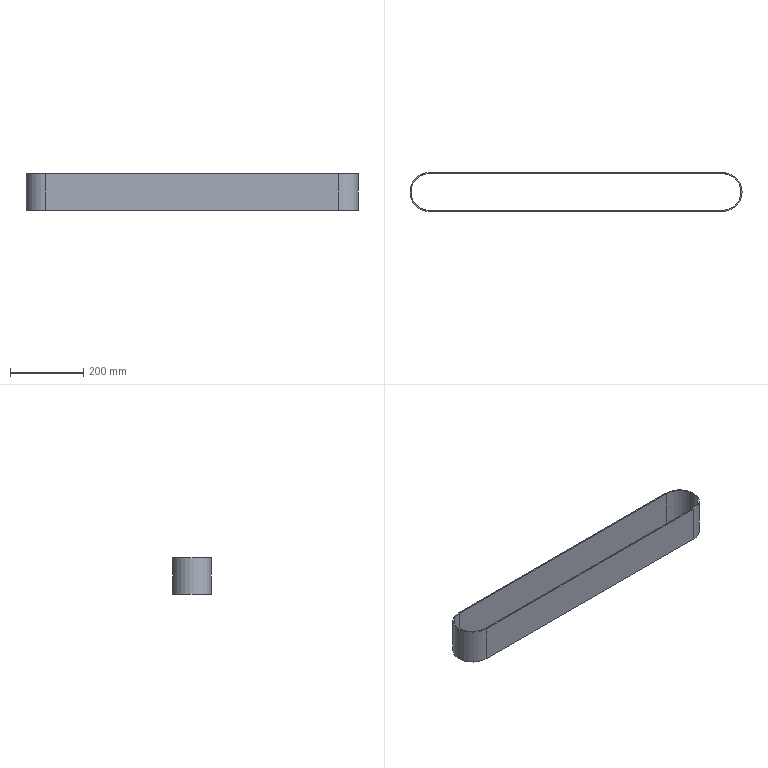Part | STEP file | 1 solid | 12 faces | box 906 x 106 x 100 mm | volume 577075 mm3 | cylinder 6 | plane 6 | commonest cylinder face diameters 100 x3 106 x3
STEP:
#1=CARTESIAN_POINT('',(0.,0.,0.));
#2=DIRECTION('',(0.,0.,1.));
#3=DIRECTION('',(1.,0.,0.));
#4=AXIS2_PLACEMENT_3D('',#1,#2,#3);
#5=CARTESIAN_POINT('',(640.53,56.408,0.));
#6=VERTEX_POINT('',#5);
#7=CARTESIAN_POINT('',(640.53,56.408,100.));
#8=VERTEX_POINT('',#7);
#9=CARTESIAN_POINT('',(640.53,56.408,0.));
#10=DIRECTION('',(0.,0.,1.));
#11=VECTOR('',#10,1.);
#12=LINE('',#9,#11);
#13=CARTESIAN_POINT('',(640.53,6.408,0.));
#14=DIRECTION('',(0.,0.,1.));
#15=DIRECTION('',(1.,0.,0.));
#16=AXIS2_PLACEMENT_3D('',#13,#14,#15);
#17=CYLINDRICAL_SURFACE('',#16,50.);
#18=CARTESIAN_POINT('',(1.571,0.));
#19=DIRECTION('',(0.,1.));
#20=VECTOR('',#19,1.);
#21=LINE('',#18,#20);
#22=(GEOMETRIC_REPRESENTATION_CONTEXT(2)PARAMETRIC_REPRESENTATION_CONTEXT()REPRESENTATION_CONTEXT('',''));
#23=DEFINITIONAL_REPRESENTATION('',(#21),#22);
#24=PCURVE('',#17,#23);
#25=CARTESIAN_POINT('',(640.53,56.408,0.));
#26=DIRECTION('',(0.,1.,0.));
#27=DIRECTION('',(0.,0.,1.));
#28=AXIS2_PLACEMENT_3D('',#25,#26,#27);
#29=PLANE('',#28);
#30=CARTESIAN_POINT('',(0.,0.));
#31=DIRECTION('',(1.,0.));
#32=VECTOR('',#31,1.);
#33=LINE('',#30,#32);
#34=(GEOMETRIC_REPRESENTATION_CONTEXT(2)PARAMETRIC_REPRESENTATION_CONTEXT()REPRESENTATION_CONTEXT('',''));
#35=DEFINITIONAL_REPRESENTATION('',(#33),#34);
#36=PCURVE('',#29,#35);
#37=SURFACE_CURVE('',#12,(#24,#36),.PCURVE_S1.);
#38=EDGE_CURVE('',#6,#8,#37,.T.);
#39=ORIENTED_EDGE('',*,*,#38,.T.);
#40=CARTESIAN_POINT('',(690.53,6.408,100.));
#41=VERTEX_POINT('',#40);
#42=CARTESIAN_POINT('',(640.53,6.408,100.));
#43=DIRECTION('',(0.,0.,-1.));
#44=DIRECTION('',(1.,0.,0.));
#45=AXIS2_PLACEMENT_3D('',#42,#43,#44);
#46=CIRCLE('',#45,50.);
#47=CARTESIAN_POINT('',(6.283,100.));
#48=DIRECTION('',(-1.,0.));
#49=VECTOR('',#48,1.);
#50=LINE('',#47,#49);
#51=(GEOMETRIC_REPRESENTATION_CONTEXT(2)PARAMETRIC_REPRESENTATION_CONTEXT()REPRESENTATION_CONTEXT('',''));
#52=DEFINITIONAL_REPRESENTATION('',(#50),#51);
#53=PCURVE('',#17,#52);
#54=CARTESIAN_POINT('',(240.531,6.408,100.));
#55=DIRECTION('',(0.,0.,1.));
#56=DIRECTION('',(1.,0.,0.));
#57=AXIS2_PLACEMENT_3D('',#54,#55,#56);
#58=PLANE('',#57);
#59=CARTESIAN_POINT('',(450.,0.));
#60=CARTESIAN_POINT('',(450.,-86.603));
#61=CARTESIAN_POINT('',(375.,-43.301));
#62=CARTESIAN_POINT('',(300.,0.));
#63=CARTESIAN_POINT('',(375.,43.301));
#64=CARTESIAN_POINT('',(450.,86.603));
#65=CARTESIAN_POINT('',(450.,0.));
#66=(BOUNDED_CURVE()B_SPLINE_CURVE(2,(#59,#60,#61,#62,#63,#64,#65),.UNSPECIFIED.,.T.,.F.)B_SPLINE_CURVE_WITH_KNOTS((1,2,2,2,2,1),(-2.094,0.,2.094,4.189,6.283,8.378),.UNSPECIFIED.)CURVE()GEOMETRIC_REPRESENTATION_ITEM()RATIONAL_B_SPLINE_CURVE((1.,0.5,1.,0.5,1.,0.5,1.))REPRESENTATION_ITEM(''));
#67=(GEOMETRIC_REPRESENTATION_CONTEXT(2)PARAMETRIC_REPRESENTATION_CONTEXT()REPRESENTATION_CONTEXT('',''));
#68=DEFINITIONAL_REPRESENTATION('',(#66),#67);
#69=PCURVE('',#58,#68);
#70=SURFACE_CURVE('',#46,(#53,#69),.PCURVE_S1.);
#71=EDGE_CURVE('',#8,#41,#70,.T.);
#72=ORIENTED_EDGE('',*,*,#71,.T.);
#73=CARTESIAN_POINT('',(690.53,6.408,0.));
#74=VERTEX_POINT('',#73);
#75=CARTESIAN_POINT('',(690.53,6.408,0.));
#76=DIRECTION('',(0.,0.,1.));
#77=VECTOR('',#76,1.);
#78=LINE('',#75,#77);
#79=CARTESIAN_POINT('',(0.,0.));
#80=DIRECTION('',(0.,1.));
#81=VECTOR('',#80,1.);
#82=LINE('',#79,#81);
#83=(GEOMETRIC_REPRESENTATION_CONTEXT(2)PARAMETRIC_REPRESENTATION_CONTEXT()REPRESENTATION_CONTEXT('',''));
#84=DEFINITIONAL_REPRESENTATION('',(#82),#83);
#85=PCURVE('',#17,#84);
#86=CARTESIAN_POINT('',(640.53,6.408,0.));
#87=DIRECTION('',(0.,0.,1.));
#88=DIRECTION('',(1.,0.,0.));
#89=AXIS2_PLACEMENT_3D('',#86,#87,#88);
#90=CYLINDRICAL_SURFACE('',#89,50.);
#91=CARTESIAN_POINT('',(6.283,0.));
#92=DIRECTION('',(0.,1.));
#93=VECTOR('',#92,1.);
#94=LINE('',#91,#93);
#95=(GEOMETRIC_REPRESENTATION_CONTEXT(2)PARAMETRIC_REPRESENTATION_CONTEXT()REPRESENTATION_CONTEXT('',''));
#96=DEFINITIONAL_REPRESENTATION('',(#94),#95);
#97=PCURVE('',#90,#96);
#98=SURFACE_CURVE('',#78,(#85,#97),.PCURVE_S1.);
#99=EDGE_CURVE('',#74,#41,#98,.T.);
#100=ORIENTED_EDGE('',*,*,#99,.F.);
#101=CARTESIAN_POINT('',(640.53,6.408,0.));
#102=DIRECTION('',(0.,0.,-1.));
#103=DIRECTION('',(1.,0.,0.));
#104=AXIS2_PLACEMENT_3D('',#101,#102,#103);
#105=CIRCLE('',#104,50.);
#106=CARTESIAN_POINT('',(6.283,0.));
#107=DIRECTION('',(-1.,0.));
#108=VECTOR('',#107,1.);
#109=LINE('',#106,#108);
#110=(GEOMETRIC_REPRESENTATION_CONTEXT(2)PARAMETRIC_REPRESENTATION_CONTEXT()REPRESENTATION_CONTEXT('',''));
#111=DEFINITIONAL_REPRESENTATION('',(#109),#110);
#112=PCURVE('',#17,#111);
#113=CARTESIAN_POINT('',(240.531,6.408,0.));
#114=DIRECTION('',(0.,0.,1.));
#115=DIRECTION('',(1.,0.,0.));
#116=AXIS2_PLACEMENT_3D('',#113,#114,#115);
#117=PLANE('',#116);
#118=CARTESIAN_POINT('',(450.,0.));
#119=CARTESIAN_POINT('',(450.,-86.603));
#120=CARTESIAN_POINT('',(375.,-43.301));
#121=CARTESIAN_POINT('',(300.,0.));
#122=CARTESIAN_POINT('',(375.,43.301));
#123=CARTESIAN_POINT('',(450.,86.603));
#124=CARTESIAN_POINT('',(450.,0.));
#125=(BOUNDED_CURVE()B_SPLINE_CURVE(2,(#118,#119,#120,#121,#122,#123,#124),.UNSPECIFIED.,.T.,.F.)B_SPLINE_CURVE_WITH_KNOTS((1,2,2,2,2,1),(-2.094,0.,2.094,4.189,6.283,8.378),.UNSPECIFIED.)CURVE()GEOMETRIC_REPRESENTATION_ITEM()RATIONAL_B_SPLINE_CURVE((1.,0.5,1.,0.5,1.,0.5,1.))REPRESENTATION_ITEM(''));
#126=(GEOMETRIC_REPRESENTATION_CONTEXT(2)PARAMETRIC_REPRESENTATION_CONTEXT()REPRESENTATION_CONTEXT('',''));
#127=DEFINITIONAL_REPRESENTATION('',(#125),#126);
#128=PCURVE('',#117,#127);
#129=SURFACE_CURVE('',#105,(#112,#128),.PCURVE_S1.);
#130=EDGE_CURVE('',#6,#74,#129,.T.);
#131=ORIENTED_EDGE('',*,*,#130,.F.);
#132=EDGE_LOOP('',(#39,#72,#100,#131));
#133=FACE_BOUND('',#132,.F.);
#134=ADVANCED_FACE('',(#133),#17,.F.);
#135=CARTESIAN_POINT('',(640.53,-46.592,0.));
#136=VERTEX_POINT('',#135);
#137=CARTESIAN_POINT('',(693.53,6.408,0.));
#138=VERTEX_POINT('',#137);
#139=CARTESIAN_POINT('',(640.53,6.408,0.));
#140=DIRECTION('',(0.,0.,1.));
#141=DIRECTION('',(1.,0.,0.));
#142=AXIS2_PLACEMENT_3D('',#139,#140,#141);
#143=CIRCLE('',#142,53.);
#144=CARTESIAN_POINT('',(640.53,6.408,0.));
#145=DIRECTION('',(0.,0.,1.));
#146=DIRECTION('',(1.,0.,0.));
#147=AXIS2_PLACEMENT_3D('',#144,#145,#146);
#148=CYLINDRICAL_SURFACE('',#147,53.);
#149=CARTESIAN_POINT('',(0.,0.));
#150=DIRECTION('',(1.,0.));
#151=VECTOR('',#150,1.);
#152=LINE('',#149,#151);
#153=(GEOMETRIC_REPRESENTATION_CONTEXT(2)PARAMETRIC_REPRESENTATION_CONTEXT()REPRESENTATION_CONTEXT('',''));
#154=DEFINITIONAL_REPRESENTATION('',(#152),#153);
#155=PCURVE('',#148,#154);
#156=CARTESIAN_POINT('',(400.,0.));
#157=DIRECTION('',(1.,0.));
#158=AXIS2_PLACEMENT_2D('',#156,#157);
#159=CIRCLE('',#158,53.);
#160=(GEOMETRIC_REPRESENTATION_CONTEXT(2)PARAMETRIC_REPRESENTATION_CONTEXT()REPRESENTATION_CONTEXT('',''));
#161=DEFINITIONAL_REPRESENTATION('',(#159),#160);
#162=PCURVE('',#117,#161);
#163=SURFACE_CURVE('',#143,(#155,#162),.PCURVE_S1.);
#164=EDGE_CURVE('',#136,#138,#163,.T.);
#165=ORIENTED_EDGE('',*,*,#164,.T.);
#166=CARTESIAN_POINT('',(693.53,6.408,100.));
#167=VERTEX_POINT('',#166);
#168=CARTESIAN_POINT('',(693.53,6.408,0.));
#169=DIRECTION('',(0.,0.,1.));
#170=VECTOR('',#169,1.);
#171=LINE('',#168,#170);
#172=CARTESIAN_POINT('',(6.283,0.));
#173=DIRECTION('',(0.,1.));
#174=VECTOR('',#173,1.);
#175=LINE('',#172,#174);
#176=(GEOMETRIC_REPRESENTATION_CONTEXT(2)PARAMETRIC_REPRESENTATION_CONTEXT()REPRESENTATION_CONTEXT('',''));
#177=DEFINITIONAL_REPRESENTATION('',(#175),#176);
#178=PCURVE('',#148,#177);
#179=CARTESIAN_POINT('',(640.53,6.408,0.));
#180=DIRECTION('',(0.,0.,1.));
#181=DIRECTION('',(1.,0.,0.));
#182=AXIS2_PLACEMENT_3D('',#179,#180,#181);
#183=CYLINDRICAL_SURFACE('',#182,53.);
#184=CARTESIAN_POINT('',(0.,0.));
#185=DIRECTION('',(0.,1.));
#186=VECTOR('',#185,1.);
#187=LINE('',#184,#186);
#188=(GEOMETRIC_REPRESENTATION_CONTEXT(2)PARAMETRIC_REPRESENTATION_CONTEXT()REPRESENTATION_CONTEXT('',''));
#189=DEFINITIONAL_REPRESENTATION('',(#187),#188);
#190=PCURVE('',#183,#189);
#191=SURFACE_CURVE('',#171,(#178,#190),.PCURVE_S1.);
#192=EDGE_CURVE('',#138,#167,#191,.T.);
#193=ORIENTED_EDGE('',*,*,#192,.T.);
#194=CARTESIAN_POINT('',(640.53,-46.592,100.));
#195=VERTEX_POINT('',#194);
#196=CARTESIAN_POINT('',(640.53,6.408,100.));
#197=DIRECTION('',(0.,0.,1.));
#198=DIRECTION('',(1.,0.,0.));
#199=AXIS2_PLACEMENT_3D('',#196,#197,#198);
#200=CIRCLE('',#199,53.);
#201=CARTESIAN_POINT('',(0.,100.));
#202=DIRECTION('',(1.,0.));
#203=VECTOR('',#202,1.);
#204=LINE('',#201,#203);
#205=(GEOMETRIC_REPRESENTATION_CONTEXT(2)PARAMETRIC_REPRESENTATION_CONTEXT()REPRESENTATION_CONTEXT('',''));
#206=DEFINITIONAL_REPRESENTATION('',(#204),#205);
#207=PCURVE('',#148,#206);
#208=CARTESIAN_POINT('',(400.,0.));
#209=DIRECTION('',(1.,0.));
#210=AXIS2_PLACEMENT_2D('',#208,#209);
#211=CIRCLE('',#210,53.);
#212=(GEOMETRIC_REPRESENTATION_CONTEXT(2)PARAMETRIC_REPRESENTATION_CONTEXT()REPRESENTATION_CONTEXT('',''));
#213=DEFINITIONAL_REPRESENTATION('',(#211),#212);
#214=PCURVE('',#58,#213);
#215=SURFACE_CURVE('',#200,(#207,#214),.PCURVE_S1.);
#216=EDGE_CURVE('',#195,#167,#215,.T.);
#217=ORIENTED_EDGE('',*,*,#216,.F.);
#218=CARTESIAN_POINT('',(640.53,-46.592,0.));
#219=DIRECTION('',(0.,0.,-1.));
#220=VECTOR('',#219,1.);
#221=LINE('',#218,#220);
#222=CARTESIAN_POINT('',(4.712,0.));
#223=DIRECTION('',(0.,-1.));
#224=VECTOR('',#223,1.);
#225=LINE('',#222,#224);
#226=(GEOMETRIC_REPRESENTATION_CONTEXT(2)PARAMETRIC_REPRESENTATION_CONTEXT()REPRESENTATION_CONTEXT('',''));
#227=DEFINITIONAL_REPRESENTATION('',(#225),#226);
#228=PCURVE('',#148,#227);
#229=CARTESIAN_POINT('',(-159.47,-46.592,0.));
#230=DIRECTION('',(0.,-1.,0.));
#231=DIRECTION('',(1.,0.,0.));
#232=AXIS2_PLACEMENT_3D('',#229,#230,#231);
#233=PLANE('',#232);
#234=CARTESIAN_POINT('',(800.,0.));
#235=DIRECTION('',(0.,-1.));
#236=VECTOR('',#235,1.);
#237=LINE('',#234,#236);
#238=(GEOMETRIC_REPRESENTATION_CONTEXT(2)PARAMETRIC_REPRESENTATION_CONTEXT()REPRESENTATION_CONTEXT('',''));
#239=DEFINITIONAL_REPRESENTATION('',(#237),#238);
#240=PCURVE('',#233,#239);
#241=SURFACE_CURVE('',#221,(#228,#240),.PCURVE_S1.);
#242=EDGE_CURVE('',#195,#136,#241,.T.);
#243=ORIENTED_EDGE('',*,*,#242,.T.);
#244=EDGE_LOOP('',(#165,#193,#217,#243));
#245=FACE_BOUND('',#244,.T.);
#246=ADVANCED_FACE('',(#245),#148,.T.);
#247=CARTESIAN_POINT('',(-159.47,-43.592,100.));
#248=VERTEX_POINT('',#247);
#249=CARTESIAN_POINT('',(-159.47,-43.592,0.));
#250=VERTEX_POINT('',#249);
#251=CARTESIAN_POINT('',(-159.47,-43.592,0.));
#252=DIRECTION('',(0.,0.,-1.));
#253=VECTOR('',#252,1.);
#254=LINE('',#251,#253);
#255=CARTESIAN_POINT('',(-159.47,-43.592,0.));
#256=DIRECTION('',(0.,-1.,0.));
#257=DIRECTION('',(1.,0.,0.));
#258=AXIS2_PLACEMENT_3D('',#255,#256,#257);
#259=PLANE('',#258);
#260=CARTESIAN_POINT('',(0.,0.));
#261=DIRECTION('',(0.,-1.));
#262=VECTOR('',#261,1.);
#263=LINE('',#260,#262);
#264=(GEOMETRIC_REPRESENTATION_CONTEXT(2)PARAMETRIC_REPRESENTATION_CONTEXT()REPRESENTATION_CONTEXT('',''));
#265=DEFINITIONAL_REPRESENTATION('',(#263),#264);
#266=PCURVE('',#259,#265);
#267=CARTESIAN_POINT('',(-159.47,6.408,0.));
#268=DIRECTION('',(0.,0.,1.));
#269=DIRECTION('',(1.,0.,0.));
#270=AXIS2_PLACEMENT_3D('',#267,#268,#269);
#271=CYLINDRICAL_SURFACE('',#270,50.);
#272=CARTESIAN_POINT('',(4.712,0.));
#273=DIRECTION('',(0.,-1.));
#274=VECTOR('',#273,1.);
#275=LINE('',#272,#274);
#276=(GEOMETRIC_REPRESENTATION_CONTEXT(2)PARAMETRIC_REPRESENTATION_CONTEXT()REPRESENTATION_CONTEXT('',''));
#277=DEFINITIONAL_REPRESENTATION('',(#275),#276);
#278=PCURVE('',#271,#277);
#279=SURFACE_CURVE('',#254,(#266,#278),.PCURVE_S1.);
#280=EDGE_CURVE('',#248,#250,#279,.T.);
#281=ORIENTED_EDGE('',*,*,#280,.F.);
#282=CARTESIAN_POINT('',(640.53,-43.592,100.));
#283=VERTEX_POINT('',#282);
#284=CARTESIAN_POINT('',(-159.47,-43.592,100.));
#285=DIRECTION('',(-1.,0.,0.));
#286=VECTOR('',#285,1.);
#287=LINE('',#284,#286);
#288=CARTESIAN_POINT('',(0.,100.));
#289=DIRECTION('',(-1.,0.));
#290=VECTOR('',#289,1.);
#291=LINE('',#288,#290);
#292=(GEOMETRIC_REPRESENTATION_CONTEXT(2)PARAMETRIC_REPRESENTATION_CONTEXT()REPRESENTATION_CONTEXT('',''));
#293=DEFINITIONAL_REPRESENTATION('',(#291),#292);
#294=PCURVE('',#259,#293);
#295=CARTESIAN_POINT('',(-400.,-50.));
#296=DIRECTION('',(-1.,0.));
#297=VECTOR('',#296,1.);
#298=LINE('',#295,#297);
#299=(GEOMETRIC_REPRESENTATION_CONTEXT(2)PARAMETRIC_REPRESENTATION_CONTEXT()REPRESENTATION_CONTEXT('',''));
#300=DEFINITIONAL_REPRESENTATION('',(#298),#299);
#301=PCURVE('',#58,#300);
#302=SURFACE_CURVE('',#287,(#294,#301),.PCURVE_S1.);
#303=EDGE_CURVE('',#283,#248,#302,.T.);
#304=ORIENTED_EDGE('',*,*,#303,.F.);
#305=CARTESIAN_POINT('',(640.53,-43.592,0.));
#306=VERTEX_POINT('',#305);
#307=CARTESIAN_POINT('',(640.53,-43.592,0.));
#308=DIRECTION('',(0.,0.,1.));
#309=VECTOR('',#308,1.);
#310=LINE('',#307,#309);
#311=CARTESIAN_POINT('',(800.,0.));
#312=DIRECTION('',(0.,1.));
#313=VECTOR('',#312,1.);
#314=LINE('',#311,#313);
#315=(GEOMETRIC_REPRESENTATION_CONTEXT(2)PARAMETRIC_REPRESENTATION_CONTEXT()REPRESENTATION_CONTEXT('',''));
#316=DEFINITIONAL_REPRESENTATION('',(#314),#315);
#317=PCURVE('',#259,#316);
#318=CARTESIAN_POINT('',(4.712,0.));
#319=DIRECTION('',(0.,1.));
#320=VECTOR('',#319,1.);
#321=LINE('',#318,#320);
#322=(GEOMETRIC_REPRESENTATION_CONTEXT(2)PARAMETRIC_REPRESENTATION_CONTEXT()REPRESENTATION_CONTEXT('',''));
#323=DEFINITIONAL_REPRESENTATION('',(#321),#322);
#324=PCURVE('',#90,#323);
#325=SURFACE_CURVE('',#310,(#317,#324),.PCURVE_S1.);
#326=EDGE_CURVE('',#306,#283,#325,.T.);
#327=ORIENTED_EDGE('',*,*,#326,.F.);
#328=CARTESIAN_POINT('',(-159.47,-43.592,0.));
#329=DIRECTION('',(1.,0.,0.));
#330=VECTOR('',#329,1.);
#331=LINE('',#328,#330);
#332=CARTESIAN_POINT('',(0.,0.));
#333=DIRECTION('',(1.,0.));
#334=VECTOR('',#333,1.);
#335=LINE('',#332,#334);
#336=(GEOMETRIC_REPRESENTATION_CONTEXT(2)PARAMETRIC_REPRESENTATION_CONTEXT()REPRESENTATION_CONTEXT('',''));
#337=DEFINITIONAL_REPRESENTATION('',(#335),#336);
#338=PCURVE('',#259,#337);
#339=CARTESIAN_POINT('',(-400.,-50.));
#340=DIRECTION('',(1.,0.));
#341=VECTOR('',#340,1.);
#342=LINE('',#339,#341);
#343=(GEOMETRIC_REPRESENTATION_CONTEXT(2)PARAMETRIC_REPRESENTATION_CONTEXT()REPRESENTATION_CONTEXT('',''));
#344=DEFINITIONAL_REPRESENTATION('',(#342),#343);
#345=PCURVE('',#117,#344);
#346=SURFACE_CURVE('',#331,(#338,#345),.PCURVE_S1.);
#347=EDGE_CURVE('',#250,#306,#346,.T.);
#348=ORIENTED_EDGE('',*,*,#347,.F.);
#349=EDGE_LOOP('',(#281,#304,#327,#348));
#350=FACE_BOUND('',#349,.T.);
#351=ADVANCED_FACE('',(#350),#259,.F.);
#352=ORIENTED_EDGE('',*,*,#164,.F.);
#353=CARTESIAN_POINT('',(-159.47,-46.592,0.));
#354=VERTEX_POINT('',#353);
#355=CARTESIAN_POINT('',(240.531,-46.592,0.));
#356=DIRECTION('',(1.,0.,0.));
#357=VECTOR('',#356,1.);
#358=LINE('',#355,#357);
#359=CARTESIAN_POINT('',(0.,-53.));
#360=DIRECTION('',(1.,0.));
#361=VECTOR('',#360,1.);
#362=LINE('',#359,#361);
#363=(GEOMETRIC_REPRESENTATION_CONTEXT(2)PARAMETRIC_REPRESENTATION_CONTEXT()REPRESENTATION_CONTEXT('',''));
#364=DEFINITIONAL_REPRESENTATION('',(#362),#363);
#365=PCURVE('',#117,#364);
#366=CARTESIAN_POINT('',(400.,0.));
#367=DIRECTION('',(1.,0.));
#368=VECTOR('',#367,1.);
#369=LINE('',#366,#368);
#370=(GEOMETRIC_REPRESENTATION_CONTEXT(2)PARAMETRIC_REPRESENTATION_CONTEXT()REPRESENTATION_CONTEXT('',''));
#371=DEFINITIONAL_REPRESENTATION('',(#369),#370);
#372=PCURVE('',#233,#371);
#373=SURFACE_CURVE('',#358,(#365,#372),.PCURVE_S1.);
#374=EDGE_CURVE('',#354,#136,#373,.T.);
#375=ORIENTED_EDGE('',*,*,#374,.F.);
#376=CARTESIAN_POINT('',(-159.47,59.408,0.));
#377=VERTEX_POINT('',#376);
#378=CARTESIAN_POINT('',(-159.47,6.408,0.));
#379=DIRECTION('',(0.,0.,1.));
#380=DIRECTION('',(1.,0.,0.));
#381=AXIS2_PLACEMENT_3D('',#378,#379,#380);
#382=CIRCLE('',#381,53.);
#383=CARTESIAN_POINT('',(-400.,0.));
#384=DIRECTION('',(1.,0.));
#385=AXIS2_PLACEMENT_2D('',#383,#384);
#386=CIRCLE('',#385,53.);
#387=(GEOMETRIC_REPRESENTATION_CONTEXT(2)PARAMETRIC_REPRESENTATION_CONTEXT()REPRESENTATION_CONTEXT('',''));
#388=DEFINITIONAL_REPRESENTATION('',(#386),#387);
#389=PCURVE('',#117,#388);
#390=CARTESIAN_POINT('',(-159.47,6.408,0.));
#391=DIRECTION('',(0.,0.,1.));
#392=DIRECTION('',(1.,0.,0.));
#393=AXIS2_PLACEMENT_3D('',#390,#391,#392);
#394=CYLINDRICAL_SURFACE('',#393,53.);
#395=CARTESIAN_POINT('',(0.,0.));
#396=DIRECTION('',(1.,0.));
#397=VECTOR('',#396,1.);
#398=LINE('',#395,#397);
#399=(GEOMETRIC_REPRESENTATION_CONTEXT(2)PARAMETRIC_REPRESENTATION_CONTEXT()REPRESENTATION_CONTEXT('',''));
#400=DEFINITIONAL_REPRESENTATION('',(#398),#399);
#401=PCURVE('',#394,#400);
#402=SURFACE_CURVE('',#382,(#389,#401),.PCURVE_S1.);
#403=EDGE_CURVE('',#377,#354,#402,.T.);
#404=ORIENTED_EDGE('',*,*,#403,.F.);
#405=CARTESIAN_POINT('',(640.53,59.408,0.));
#406=VERTEX_POINT('',#405);
#407=CARTESIAN_POINT('',(240.531,59.408,0.));
#408=DIRECTION('',(-1.,0.,0.));
#409=VECTOR('',#408,1.);
#410=LINE('',#407,#409);
#411=CARTESIAN_POINT('',(0.,53.));
#412=DIRECTION('',(-1.,0.));
#413=VECTOR('',#412,1.);
#414=LINE('',#411,#413);
#415=(GEOMETRIC_REPRESENTATION_CONTEXT(2)PARAMETRIC_REPRESENTATION_CONTEXT()REPRESENTATION_CONTEXT('',''));
#416=DEFINITIONAL_REPRESENTATION('',(#414),#415);
#417=PCURVE('',#117,#416);
#418=CARTESIAN_POINT('',(640.53,59.408,0.));
#419=DIRECTION('',(0.,1.,0.));
#420=DIRECTION('',(-1.,0.,0.));
#421=AXIS2_PLACEMENT_3D('',#418,#419,#420);
#422=PLANE('',#421);
#423=CARTESIAN_POINT('',(400.,0.));
#424=DIRECTION('',(1.,0.));
#425=VECTOR('',#424,1.);
#426=LINE('',#423,#425);
#427=(GEOMETRIC_REPRESENTATION_CONTEXT(2)PARAMETRIC_REPRESENTATION_CONTEXT()REPRESENTATION_CONTEXT('',''));
#428=DEFINITIONAL_REPRESENTATION('',(#426),#427);
#429=PCURVE('',#422,#428);
#430=SURFACE_CURVE('',#410,(#417,#429),.PCURVE_S1.);
#431=EDGE_CURVE('',#406,#377,#430,.T.);
#432=ORIENTED_EDGE('',*,*,#431,.F.);
#433=CARTESIAN_POINT('',(640.53,6.408,0.));
#434=DIRECTION('',(0.,0.,1.));
#435=DIRECTION('',(1.,0.,0.));
#436=AXIS2_PLACEMENT_3D('',#433,#434,#435);
#437=CIRCLE('',#436,53.);
#438=CARTESIAN_POINT('',(400.,0.));
#439=DIRECTION('',(1.,0.));
#440=AXIS2_PLACEMENT_2D('',#438,#439);
#441=CIRCLE('',#440,53.);
#442=(GEOMETRIC_REPRESENTATION_CONTEXT(2)PARAMETRIC_REPRESENTATION_CONTEXT()REPRESENTATION_CONTEXT('',''));
#443=DEFINITIONAL_REPRESENTATION('',(#441),#442);
#444=PCURVE('',#117,#443);
#445=CARTESIAN_POINT('',(0.,0.));
#446=DIRECTION('',(1.,0.));
#447=VECTOR('',#446,1.);
#448=LINE('',#445,#447);
#449=(GEOMETRIC_REPRESENTATION_CONTEXT(2)PARAMETRIC_REPRESENTATION_CONTEXT()REPRESENTATION_CONTEXT('',''));
#450=DEFINITIONAL_REPRESENTATION('',(#448),#449);
#451=PCURVE('',#183,#450);
#452=SURFACE_CURVE('',#437,(#444,#451),.PCURVE_S1.);
#453=EDGE_CURVE('',#138,#406,#452,.T.);
#454=ORIENTED_EDGE('',*,*,#453,.F.);
#455=EDGE_LOOP('',(#352,#375,#404,#432,#454));
#456=FACE_BOUND('',#455,.T.);
#457=CARTESIAN_POINT('',(-159.47,56.408,0.));
#458=VERTEX_POINT('',#457);
#459=CARTESIAN_POINT('',(240.531,56.408,0.));
#460=DIRECTION('',(1.,0.,0.));
#461=VECTOR('',#460,1.);
#462=LINE('',#459,#461);
#463=CARTESIAN_POINT('',(0.,50.));
#464=DIRECTION('',(1.,0.));
#465=VECTOR('',#464,1.);
#466=LINE('',#463,#465);
#467=(GEOMETRIC_REPRESENTATION_CONTEXT(2)PARAMETRIC_REPRESENTATION_CONTEXT()REPRESENTATION_CONTEXT('',''));
#468=DEFINITIONAL_REPRESENTATION('',(#466),#467);
#469=PCURVE('',#117,#468);
#470=CARTESIAN_POINT('',(0.,-400.));
#471=DIRECTION('',(0.,1.));
#472=VECTOR('',#471,1.);
#473=LINE('',#470,#472);
#474=(GEOMETRIC_REPRESENTATION_CONTEXT(2)PARAMETRIC_REPRESENTATION_CONTEXT()REPRESENTATION_CONTEXT('',''));
#475=DEFINITIONAL_REPRESENTATION('',(#473),#474);
#476=PCURVE('',#29,#475);
#477=SURFACE_CURVE('',#462,(#469,#476),.PCURVE_S1.);
#478=EDGE_CURVE('',#458,#6,#477,.T.);
#479=ORIENTED_EDGE('',*,*,#478,.F.);
#480=CARTESIAN_POINT('',(-159.47,6.408,0.));
#481=DIRECTION('',(0.,0.,-1.));
#482=DIRECTION('',(1.,0.,0.));
#483=AXIS2_PLACEMENT_3D('',#480,#481,#482);
#484=CIRCLE('',#483,50.);
#485=CARTESIAN_POINT('',(-350.,0.));
#486=CARTESIAN_POINT('',(-350.,-86.603));
#487=CARTESIAN_POINT('',(-425.,-43.301));
#488=CARTESIAN_POINT('',(-500.,0.));
#489=CARTESIAN_POINT('',(-425.,43.301));
#490=CARTESIAN_POINT('',(-350.,86.603));
#491=CARTESIAN_POINT('',(-350.,0.));
#492=(BOUNDED_CURVE()B_SPLINE_CURVE(2,(#485,#486,#487,#488,#489,#490,#491),.UNSPECIFIED.,.T.,.F.)B_SPLINE_CURVE_WITH_KNOTS((1,2,2,2,2,1),(-2.094,0.,2.094,4.189,6.283,8.378),.UNSPECIFIED.)CURVE()GEOMETRIC_REPRESENTATION_ITEM()RATIONAL_B_SPLINE_CURVE((1.,0.5,1.,0.5,1.,0.5,1.))REPRESENTATION_ITEM(''));
#493=(GEOMETRIC_REPRESENTATION_CONTEXT(2)PARAMETRIC_REPRESENTATION_CONTEXT()REPRESENTATION_CONTEXT('',''));
#494=DEFINITIONAL_REPRESENTATION('',(#492),#493);
#495=PCURVE('',#117,#494);
#496=CARTESIAN_POINT('',(6.283,0.));
#497=DIRECTION('',(-1.,0.));
#498=VECTOR('',#497,1.);
#499=LINE('',#496,#498);
#500=(GEOMETRIC_REPRESENTATION_CONTEXT(2)PARAMETRIC_REPRESENTATION_CONTEXT()REPRESENTATION_CONTEXT('',''));
#501=DEFINITIONAL_REPRESENTATION('',(#499),#500);
#502=PCURVE('',#271,#501);
#503=SURFACE_CURVE('',#484,(#495,#502),.PCURVE_S1.);
#504=EDGE_CURVE('',#250,#458,#503,.T.);
#505=ORIENTED_EDGE('',*,*,#504,.F.);
#506=ORIENTED_EDGE('',*,*,#347,.T.);
#507=CARTESIAN_POINT('',(640.53,6.408,0.));
#508=DIRECTION('',(0.,0.,-1.));
#509=DIRECTION('',(1.,0.,0.));
#510=AXIS2_PLACEMENT_3D('',#507,#508,#509);
#511=CIRCLE('',#510,50.);
#512=CARTESIAN_POINT('',(450.,0.));
#513=CARTESIAN_POINT('',(450.,-86.603));
#514=CARTESIAN_POINT('',(375.,-43.301));
#515=CARTESIAN_POINT('',(300.,0.));
#516=CARTESIAN_POINT('',(375.,43.301));
#517=CARTESIAN_POINT('',(450.,86.603));
#518=CARTESIAN_POINT('',(450.,0.));
#519=(BOUNDED_CURVE()B_SPLINE_CURVE(2,(#512,#513,#514,#515,#516,#517,#518),.UNSPECIFIED.,.T.,.F.)B_SPLINE_CURVE_WITH_KNOTS((1,2,2,2,2,1),(-2.094,0.,2.094,4.189,6.283,8.378),.UNSPECIFIED.)CURVE()GEOMETRIC_REPRESENTATION_ITEM()RATIONAL_B_SPLINE_CURVE((1.,0.5,1.,0.5,1.,0.5,1.))REPRESENTATION_ITEM(''));
#520=(GEOMETRIC_REPRESENTATION_CONTEXT(2)PARAMETRIC_REPRESENTATION_CONTEXT()REPRESENTATION_CONTEXT('',''));
#521=DEFINITIONAL_REPRESENTATION('',(#519),#520);
#522=PCURVE('',#117,#521);
#523=CARTESIAN_POINT('',(6.283,0.));
#524=DIRECTION('',(-1.,0.));
#525=VECTOR('',#524,1.);
#526=LINE('',#523,#525);
#527=(GEOMETRIC_REPRESENTATION_CONTEXT(2)PARAMETRIC_REPRESENTATION_CONTEXT()REPRESENTATION_CONTEXT('',''));
#528=DEFINITIONAL_REPRESENTATION('',(#526),#527);
#529=PCURVE('',#90,#528);
#530=SURFACE_CURVE('',#511,(#522,#529),.PCURVE_S1.);
#531=EDGE_CURVE('',#74,#306,#530,.T.);
#532=ORIENTED_EDGE('',*,*,#531,.F.);
#533=ORIENTED_EDGE('',*,*,#130,.F.);
#534=EDGE_LOOP('',(#479,#505,#506,#532,#533));
#535=FACE_BOUND('',#534,.T.);
#536=ADVANCED_FACE('',(#456,#535),#117,.F.);
#537=ORIENTED_EDGE('',*,*,#504,.F.);
#538=ORIENTED_EDGE('',*,*,#280,.F.);
#539=CARTESIAN_POINT('',(-159.47,56.408,100.));
#540=VERTEX_POINT('',#539);
#541=CARTESIAN_POINT('',(-159.47,6.408,100.));
#542=DIRECTION('',(0.,0.,-1.));
#543=DIRECTION('',(1.,0.,0.));
#544=AXIS2_PLACEMENT_3D('',#541,#542,#543);
#545=CIRCLE('',#544,50.);
#546=CARTESIAN_POINT('',(6.283,100.));
#547=DIRECTION('',(-1.,0.));
#548=VECTOR('',#547,1.);
#549=LINE('',#546,#548);
#550=(GEOMETRIC_REPRESENTATION_CONTEXT(2)PARAMETRIC_REPRESENTATION_CONTEXT()REPRESENTATION_CONTEXT('',''));
#551=DEFINITIONAL_REPRESENTATION('',(#549),#550);
#552=PCURVE('',#271,#551);
#553=CARTESIAN_POINT('',(-350.,0.));
#554=CARTESIAN_POINT('',(-350.,-86.603));
#555=CARTESIAN_POINT('',(-425.,-43.301));
#556=CARTESIAN_POINT('',(-500.,0.));
#557=CARTESIAN_POINT('',(-425.,43.301));
#558=CARTESIAN_POINT('',(-350.,86.603));
#559=CARTESIAN_POINT('',(-350.,0.));
#560=(BOUNDED_CURVE()B_SPLINE_CURVE(2,(#553,#554,#555,#556,#557,#558,#559),.UNSPECIFIED.,.T.,.F.)B_SPLINE_CURVE_WITH_KNOTS((1,2,2,2,2,1),(-2.094,0.,2.094,4.189,6.283,8.378),.UNSPECIFIED.)CURVE()GEOMETRIC_REPRESENTATION_ITEM()RATIONAL_B_SPLINE_CURVE((1.,0.5,1.,0.5,1.,0.5,1.))REPRESENTATION_ITEM(''));
#561=(GEOMETRIC_REPRESENTATION_CONTEXT(2)PARAMETRIC_REPRESENTATION_CONTEXT()REPRESENTATION_CONTEXT('',''));
#562=DEFINITIONAL_REPRESENTATION('',(#560),#561);
#563=PCURVE('',#58,#562);
#564=SURFACE_CURVE('',#545,(#552,#563),.PCURVE_S1.);
#565=EDGE_CURVE('',#248,#540,#564,.T.);
#566=ORIENTED_EDGE('',*,*,#565,.T.);
#567=CARTESIAN_POINT('',(-159.47,56.408,0.));
#568=DIRECTION('',(0.,0.,-1.));
#569=VECTOR('',#568,1.);
#570=LINE('',#567,#569);
#571=CARTESIAN_POINT('',(1.571,0.));
#572=DIRECTION('',(0.,-1.));
#573=VECTOR('',#572,1.);
#574=LINE('',#571,#573);
#575=(GEOMETRIC_REPRESENTATION_CONTEXT(2)PARAMETRIC_REPRESENTATION_CONTEXT()REPRESENTATION_CONTEXT('',''));
#576=DEFINITIONAL_REPRESENTATION('',(#574),#575);
#577=PCURVE('',#271,#576);
#578=CARTESIAN_POINT('',(0.,-800.));
#579=DIRECTION('',(-1.,0.));
#580=VECTOR('',#579,1.);
#581=LINE('',#578,#580);
#582=(GEOMETRIC_REPRESENTATION_CONTEXT(2)PARAMETRIC_REPRESENTATION_CONTEXT()REPRESENTATION_CONTEXT('',''));
#583=DEFINITIONAL_REPRESENTATION('',(#581),#582);
#584=PCURVE('',#29,#583);
#585=SURFACE_CURVE('',#570,(#577,#584),.PCURVE_S1.);
#586=EDGE_CURVE('',#540,#458,#585,.T.);
#587=ORIENTED_EDGE('',*,*,#586,.T.);
#588=EDGE_LOOP('',(#537,#538,#566,#587));
#589=FACE_BOUND('',#588,.F.);
#590=ADVANCED_FACE('',(#589),#271,.F.);
#591=CARTESIAN_POINT('',(-159.47,-46.592,100.));
#592=VERTEX_POINT('',#591);
#593=CARTESIAN_POINT('',(240.531,-46.592,100.));
#594=DIRECTION('',(1.,0.,0.));
#595=VECTOR('',#594,1.);
#596=LINE('',#593,#595);
#597=CARTESIAN_POINT('',(0.,-53.));
#598=DIRECTION('',(1.,0.));
#599=VECTOR('',#598,1.);
#600=LINE('',#597,#599);
#601=(GEOMETRIC_REPRESENTATION_CONTEXT(2)PARAMETRIC_REPRESENTATION_CONTEXT()REPRESENTATION_CONTEXT('',''));
#602=DEFINITIONAL_REPRESENTATION('',(#600),#601);
#603=PCURVE('',#58,#602);
#604=CARTESIAN_POINT('',(400.,100.));
#605=DIRECTION('',(1.,0.));
#606=VECTOR('',#605,1.);
#607=LINE('',#604,#606);
#608=(GEOMETRIC_REPRESENTATION_CONTEXT(2)PARAMETRIC_REPRESENTATION_CONTEXT()REPRESENTATION_CONTEXT('',''));
#609=DEFINITIONAL_REPRESENTATION('',(#607),#608);
#610=PCURVE('',#233,#609);
#611=SURFACE_CURVE('',#596,(#603,#610),.PCURVE_S1.);
#612=EDGE_CURVE('',#592,#195,#611,.T.);
#613=ORIENTED_EDGE('',*,*,#612,.T.);
#614=ORIENTED_EDGE('',*,*,#216,.T.);
#615=CARTESIAN_POINT('',(640.53,59.408,100.));
#616=VERTEX_POINT('',#615);
#617=CARTESIAN_POINT('',(640.53,6.408,100.));
#618=DIRECTION('',(0.,0.,1.));
#619=DIRECTION('',(1.,0.,0.));
#620=AXIS2_PLACEMENT_3D('',#617,#618,#619);
#621=CIRCLE('',#620,53.);
#622=CARTESIAN_POINT('',(400.,0.));
#623=DIRECTION('',(1.,0.));
#624=AXIS2_PLACEMENT_2D('',#622,#623);
#625=CIRCLE('',#624,53.);
#626=(GEOMETRIC_REPRESENTATION_CONTEXT(2)PARAMETRIC_REPRESENTATION_CONTEXT()REPRESENTATION_CONTEXT('',''));
#627=DEFINITIONAL_REPRESENTATION('',(#625),#626);
#628=PCURVE('',#58,#627);
#629=CARTESIAN_POINT('',(0.,100.));
#630=DIRECTION('',(1.,0.));
#631=VECTOR('',#630,1.);
#632=LINE('',#629,#631);
#633=(GEOMETRIC_REPRESENTATION_CONTEXT(2)PARAMETRIC_REPRESENTATION_CONTEXT()REPRESENTATION_CONTEXT('',''));
#634=DEFINITIONAL_REPRESENTATION('',(#632),#633);
#635=PCURVE('',#183,#634);
#636=SURFACE_CURVE('',#621,(#628,#635),.PCURVE_S1.);
#637=EDGE_CURVE('',#167,#616,#636,.T.);
#638=ORIENTED_EDGE('',*,*,#637,.T.);
#639=CARTESIAN_POINT('',(-159.47,59.408,100.));
#640=VERTEX_POINT('',#639);
#641=CARTESIAN_POINT('',(240.531,59.408,100.));
#642=DIRECTION('',(-1.,0.,0.));
#643=VECTOR('',#642,1.);
#644=LINE('',#641,#643);
#645=CARTESIAN_POINT('',(0.,53.));
#646=DIRECTION('',(-1.,0.));
#647=VECTOR('',#646,1.);
#648=LINE('',#645,#647);
#649=(GEOMETRIC_REPRESENTATION_CONTEXT(2)PARAMETRIC_REPRESENTATION_CONTEXT()REPRESENTATION_CONTEXT('',''));
#650=DEFINITIONAL_REPRESENTATION('',(#648),#649);
#651=PCURVE('',#58,#650);
#652=CARTESIAN_POINT('',(400.,100.));
#653=DIRECTION('',(1.,0.));
#654=VECTOR('',#653,1.);
#655=LINE('',#652,#654);
#656=(GEOMETRIC_REPRESENTATION_CONTEXT(2)PARAMETRIC_REPRESENTATION_CONTEXT()REPRESENTATION_CONTEXT('',''));
#657=DEFINITIONAL_REPRESENTATION('',(#655),#656);
#658=PCURVE('',#422,#657);
#659=SURFACE_CURVE('',#644,(#651,#658),.PCURVE_S1.);
#660=EDGE_CURVE('',#616,#640,#659,.T.);
#661=ORIENTED_EDGE('',*,*,#660,.T.);
#662=CARTESIAN_POINT('',(-159.47,6.408,100.));
#663=DIRECTION('',(0.,0.,1.));
#664=DIRECTION('',(1.,0.,0.));
#665=AXIS2_PLACEMENT_3D('',#662,#663,#664);
#666=CIRCLE('',#665,53.);
#667=CARTESIAN_POINT('',(-400.,0.));
#668=DIRECTION('',(1.,0.));
#669=AXIS2_PLACEMENT_2D('',#667,#668);
#670=CIRCLE('',#669,53.);
#671=(GEOMETRIC_REPRESENTATION_CONTEXT(2)PARAMETRIC_REPRESENTATION_CONTEXT()REPRESENTATION_CONTEXT('',''));
#672=DEFINITIONAL_REPRESENTATION('',(#670),#671);
#673=PCURVE('',#58,#672);
#674=CARTESIAN_POINT('',(0.,100.));
#675=DIRECTION('',(1.,0.));
#676=VECTOR('',#675,1.);
#677=LINE('',#674,#676);
#678=(GEOMETRIC_REPRESENTATION_CONTEXT(2)PARAMETRIC_REPRESENTATION_CONTEXT()REPRESENTATION_CONTEXT('',''));
#679=DEFINITIONAL_REPRESENTATION('',(#677),#678);
#680=PCURVE('',#394,#679);
#681=SURFACE_CURVE('',#666,(#673,#680),.PCURVE_S1.);
#682=EDGE_CURVE('',#640,#592,#681,.T.);
#683=ORIENTED_EDGE('',*,*,#682,.T.);
#684=EDGE_LOOP('',(#613,#614,#638,#661,#683));
#685=FACE_BOUND('',#684,.T.);
#686=ORIENTED_EDGE('',*,*,#565,.T.);
#687=CARTESIAN_POINT('',(240.531,56.408,100.));
#688=DIRECTION('',(1.,0.,0.));
#689=VECTOR('',#688,1.);
#690=LINE('',#687,#689);
#691=CARTESIAN_POINT('',(0.,50.));
#692=DIRECTION('',(1.,0.));
#693=VECTOR('',#692,1.);
#694=LINE('',#691,#693);
#695=(GEOMETRIC_REPRESENTATION_CONTEXT(2)PARAMETRIC_REPRESENTATION_CONTEXT()REPRESENTATION_CONTEXT('',''));
#696=DEFINITIONAL_REPRESENTATION('',(#694),#695);
#697=PCURVE('',#58,#696);
#698=CARTESIAN_POINT('',(100.,-400.));
#699=DIRECTION('',(0.,1.));
#700=VECTOR('',#699,1.);
#701=LINE('',#698,#700);
#702=(GEOMETRIC_REPRESENTATION_CONTEXT(2)PARAMETRIC_REPRESENTATION_CONTEXT()REPRESENTATION_CONTEXT('',''));
#703=DEFINITIONAL_REPRESENTATION('',(#701),#702);
#704=PCURVE('',#29,#703);
#705=SURFACE_CURVE('',#690,(#697,#704),.PCURVE_S1.);
#706=EDGE_CURVE('',#540,#8,#705,.T.);
#707=ORIENTED_EDGE('',*,*,#706,.T.);
#708=ORIENTED_EDGE('',*,*,#71,.T.);
#709=CARTESIAN_POINT('',(640.53,6.408,100.));
#710=DIRECTION('',(0.,0.,-1.));
#711=DIRECTION('',(1.,0.,0.));
#712=AXIS2_PLACEMENT_3D('',#709,#710,#711);
#713=CIRCLE('',#712,50.);
#714=CARTESIAN_POINT('',(450.,0.));
#715=CARTESIAN_POINT('',(450.,-86.603));
#716=CARTESIAN_POINT('',(375.,-43.301));
#717=CARTESIAN_POINT('',(300.,0.));
#718=CARTESIAN_POINT('',(375.,43.301));
#719=CARTESIAN_POINT('',(450.,86.603));
#720=CARTESIAN_POINT('',(450.,0.));
#721=(BOUNDED_CURVE()B_SPLINE_CURVE(2,(#714,#715,#716,#717,#718,#719,#720),.UNSPECIFIED.,.T.,.F.)B_SPLINE_CURVE_WITH_KNOTS((1,2,2,2,2,1),(-2.094,0.,2.094,4.189,6.283,8.378),.UNSPECIFIED.)CURVE()GEOMETRIC_REPRESENTATION_ITEM()RATIONAL_B_SPLINE_CURVE((1.,0.5,1.,0.5,1.,0.5,1.))REPRESENTATION_ITEM(''));
#722=(GEOMETRIC_REPRESENTATION_CONTEXT(2)PARAMETRIC_REPRESENTATION_CONTEXT()REPRESENTATION_CONTEXT('',''));
#723=DEFINITIONAL_REPRESENTATION('',(#721),#722);
#724=PCURVE('',#58,#723);
#725=CARTESIAN_POINT('',(6.283,100.));
#726=DIRECTION('',(-1.,0.));
#727=VECTOR('',#726,1.);
#728=LINE('',#725,#727);
#729=(GEOMETRIC_REPRESENTATION_CONTEXT(2)PARAMETRIC_REPRESENTATION_CONTEXT()REPRESENTATION_CONTEXT('',''));
#730=DEFINITIONAL_REPRESENTATION('',(#728),#729);
#731=PCURVE('',#90,#730);
#732=SURFACE_CURVE('',#713,(#724,#731),.PCURVE_S1.);
#733=EDGE_CURVE('',#41,#283,#732,.T.);
#734=ORIENTED_EDGE('',*,*,#733,.T.);
#735=ORIENTED_EDGE('',*,*,#303,.T.);
#736=EDGE_LOOP('',(#686,#707,#708,#734,#735));
#737=FACE_BOUND('',#736,.T.);
#738=ADVANCED_FACE('',(#685,#737),#58,.T.);
#739=ORIENTED_EDGE('',*,*,#733,.T.);
#740=ORIENTED_EDGE('',*,*,#326,.F.);
#741=ORIENTED_EDGE('',*,*,#531,.F.);
#742=ORIENTED_EDGE('',*,*,#99,.T.);
#743=EDGE_LOOP('',(#739,#740,#741,#742));
#744=FACE_BOUND('',#743,.F.);
#745=ADVANCED_FACE('',(#744),#90,.F.);
#746=ORIENTED_EDGE('',*,*,#660,.F.);
#747=CARTESIAN_POINT('',(640.53,59.408,0.));
#748=DIRECTION('',(0.,0.,-1.));
#749=VECTOR('',#748,1.);
#750=LINE('',#747,#749);
#751=CARTESIAN_POINT('',(0.,0.));
#752=DIRECTION('',(0.,-1.));
#753=VECTOR('',#752,1.);
#754=LINE('',#751,#753);
#755=(GEOMETRIC_REPRESENTATION_CONTEXT(2)PARAMETRIC_REPRESENTATION_CONTEXT()REPRESENTATION_CONTEXT('',''));
#756=DEFINITIONAL_REPRESENTATION('',(#754),#755);
#757=PCURVE('',#422,#756);
#758=CARTESIAN_POINT('',(1.571,0.));
#759=DIRECTION('',(0.,-1.));
#760=VECTOR('',#759,1.);
#761=LINE('',#758,#760);
#762=(GEOMETRIC_REPRESENTATION_CONTEXT(2)PARAMETRIC_REPRESENTATION_CONTEXT()REPRESENTATION_CONTEXT('',''));
#763=DEFINITIONAL_REPRESENTATION('',(#761),#762);
#764=PCURVE('',#183,#763);
#765=SURFACE_CURVE('',#750,(#757,#764),.PCURVE_S1.);
#766=EDGE_CURVE('',#616,#406,#765,.T.);
#767=ORIENTED_EDGE('',*,*,#766,.T.);
#768=ORIENTED_EDGE('',*,*,#431,.T.);
#769=CARTESIAN_POINT('',(-159.47,59.408,0.));
#770=DIRECTION('',(0.,0.,1.));
#771=VECTOR('',#770,1.);
#772=LINE('',#769,#771);
#773=CARTESIAN_POINT('',(800.,0.));
#774=DIRECTION('',(0.,1.));
#775=VECTOR('',#774,1.);
#776=LINE('',#773,#775);
#777=(GEOMETRIC_REPRESENTATION_CONTEXT(2)PARAMETRIC_REPRESENTATION_CONTEXT()REPRESENTATION_CONTEXT('',''));
#778=DEFINITIONAL_REPRESENTATION('',(#776),#777);
#779=PCURVE('',#422,#778);
#780=CARTESIAN_POINT('',(1.571,0.));
#781=DIRECTION('',(0.,1.));
#782=VECTOR('',#781,1.);
#783=LINE('',#780,#782);
#784=(GEOMETRIC_REPRESENTATION_CONTEXT(2)PARAMETRIC_REPRESENTATION_CONTEXT()REPRESENTATION_CONTEXT('',''));
#785=DEFINITIONAL_REPRESENTATION('',(#783),#784);
#786=PCURVE('',#394,#785);
#787=SURFACE_CURVE('',#772,(#779,#786),.PCURVE_S1.);
#788=EDGE_CURVE('',#377,#640,#787,.T.);
#789=ORIENTED_EDGE('',*,*,#788,.T.);
#790=EDGE_LOOP('',(#746,#767,#768,#789));
#791=FACE_BOUND('',#790,.T.);
#792=ADVANCED_FACE('',(#791),#422,.T.);
#793=ORIENTED_EDGE('',*,*,#192,.F.);
#794=ORIENTED_EDGE('',*,*,#453,.T.);
#795=ORIENTED_EDGE('',*,*,#766,.F.);
#796=ORIENTED_EDGE('',*,*,#637,.F.);
#797=EDGE_LOOP('',(#793,#794,#795,#796));
#798=FACE_BOUND('',#797,.T.);
#799=ADVANCED_FACE('',(#798),#183,.T.);
#800=ORIENTED_EDGE('',*,*,#612,.F.);
#801=CARTESIAN_POINT('',(-159.47,-46.592,0.));
#802=DIRECTION('',(0.,0.,-1.));
#803=VECTOR('',#802,1.);
#804=LINE('',#801,#803);
#805=CARTESIAN_POINT('',(0.,0.));
#806=DIRECTION('',(0.,-1.));
#807=VECTOR('',#806,1.);
#808=LINE('',#805,#807);
#809=(GEOMETRIC_REPRESENTATION_CONTEXT(2)PARAMETRIC_REPRESENTATION_CONTEXT()REPRESENTATION_CONTEXT('',''));
#810=DEFINITIONAL_REPRESENTATION('',(#808),#809);
#811=PCURVE('',#233,#810);
#812=CARTESIAN_POINT('',(4.712,0.));
#813=DIRECTION('',(0.,-1.));
#814=VECTOR('',#813,1.);
#815=LINE('',#812,#814);
#816=(GEOMETRIC_REPRESENTATION_CONTEXT(2)PARAMETRIC_REPRESENTATION_CONTEXT()REPRESENTATION_CONTEXT('',''));
#817=DEFINITIONAL_REPRESENTATION('',(#815),#816);
#818=PCURVE('',#394,#817);
#819=SURFACE_CURVE('',#804,(#811,#818),.PCURVE_S1.);
#820=EDGE_CURVE('',#592,#354,#819,.T.);
#821=ORIENTED_EDGE('',*,*,#820,.T.);
#822=ORIENTED_EDGE('',*,*,#374,.T.);
#823=ORIENTED_EDGE('',*,*,#242,.F.);
#824=EDGE_LOOP('',(#800,#821,#822,#823));
#825=FACE_BOUND('',#824,.T.);
#826=ADVANCED_FACE('',(#825),#233,.T.);
#827=ORIENTED_EDGE('',*,*,#682,.F.);
#828=ORIENTED_EDGE('',*,*,#788,.F.);
#829=ORIENTED_EDGE('',*,*,#403,.T.);
#830=ORIENTED_EDGE('',*,*,#820,.F.);
#831=EDGE_LOOP('',(#827,#828,#829,#830));
#832=FACE_BOUND('',#831,.T.);
#833=ADVANCED_FACE('',(#832),#394,.T.);
#834=ORIENTED_EDGE('',*,*,#38,.T.);
#835=ORIENTED_EDGE('',*,*,#706,.F.);
#836=ORIENTED_EDGE('',*,*,#586,.T.);
#837=ORIENTED_EDGE('',*,*,#478,.T.);
#838=EDGE_LOOP('',(#834,#835,#836,#837));
#839=FACE_BOUND('',#838,.T.);
#840=ADVANCED_FACE('',(#839),#29,.F.);
#841=CLOSED_SHELL('',(#134,#246,#351,#536,#590,#738,#745,#792,#799,#826,#833,#840));
#842=MANIFOLD_SOLID_BREP('',#841);
#843=(LENGTH_UNIT()NAMED_UNIT(*)SI_UNIT(.MILLI.,.METRE.));
#844=UNCERTAINTY_MEASURE_WITH_UNIT(LENGTH_MEASURE(0.0000001),#843,'','');
#845=(NAMED_UNIT(*)PLANE_ANGLE_UNIT()SI_UNIT($,.RADIAN.));
#846=(NAMED_UNIT(*)SI_UNIT($,.STERADIAN.)SOLID_ANGLE_UNIT());
#847=(GEOMETRIC_REPRESENTATION_CONTEXT(3)GLOBAL_UNCERTAINTY_ASSIGNED_CONTEXT((#844))GLOBAL_UNIT_ASSIGNED_CONTEXT((#843,#845,#846))REPRESENTATION_CONTEXT('',''));
#848=ADVANCED_BREP_SHAPE_REPRESENTATION('',(#4,#842),#847);